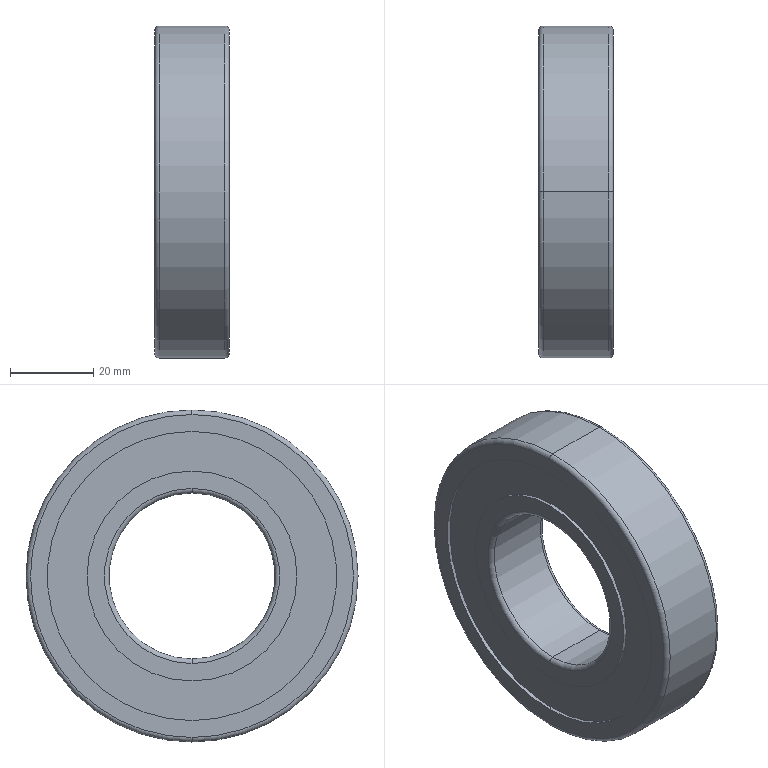Part | SolidWorks | features Fillet 2, Revolution 1 | 1 solid | 26 faces | box 18 x 80 x 80 mm | volume 64676 mm3 | cylinder 12 | torus 8 | plane 6 | commonest cylinder face diameters 50.6 x4 69.65 x4 40 x2 80 x2
STEP:
#1=CARTESIAN_POINT('',(1.1,0.,20.));
#2=VERTEX_POINT('',#1);
#3=CARTESIAN_POINT('',(1.1,0.,-20.));
#4=VERTEX_POINT('',#3);
#5=CARTESIAN_POINT('',(1.1,0.,0.));
#6=DIRECTION('',(-1.,0.,0.));
#7=DIRECTION('',(0.,0.,-1.));
#8=AXIS2_PLACEMENT_3D('',#5,#6,#7);
#9=CIRCLE('',#8,20.);
#10=EDGE_CURVE('',#2,#4,#9,.T.);
#11=ORIENTED_EDGE('',*,*,#10,.F.);
#12=CARTESIAN_POINT('',(0.,0.,21.1));
#13=VERTEX_POINT('',#12);
#14=CARTESIAN_POINT('',(1.1,0.,21.1));
#15=DIRECTION('',(0.,1.,0.));
#16=DIRECTION('',(0.,0.,1.));
#17=AXIS2_PLACEMENT_3D('',#14,#15,#16);
#18=CIRCLE('',#17,1.1);
#19=EDGE_CURVE('',#2,#13,#18,.T.);
#20=ORIENTED_EDGE('',*,*,#19,.T.);
#21=CARTESIAN_POINT('',(0.,0.,-21.1));
#22=VERTEX_POINT('',#21);
#23=CARTESIAN_POINT('',(0.,0.,0.));
#24=DIRECTION('',(1.,0.,0.));
#25=DIRECTION('',(0.,0.,-1.));
#26=AXIS2_PLACEMENT_3D('',#23,#24,#25);
#27=CIRCLE('',#26,21.1);
#28=EDGE_CURVE('',#22,#13,#27,.T.);
#29=ORIENTED_EDGE('',*,*,#28,.F.);
#30=CARTESIAN_POINT('',(1.1,0.,-21.1));
#31=DIRECTION('',(0.,-1.,0.));
#32=DIRECTION('',(0.,0.,-1.));
#33=AXIS2_PLACEMENT_3D('',#30,#31,#32);
#34=CIRCLE('',#33,1.1);
#35=EDGE_CURVE('',#4,#22,#34,.T.);
#36=ORIENTED_EDGE('',*,*,#35,.F.);
#37=EDGE_LOOP('',(#11,#20,#29,#36));
#38=FACE_OUTER_BOUND('',#37,.T.);
#39=CARTESIAN_POINT('',(1.1,0.,0.));
#40=DIRECTION('',(1.,0.,0.));
#41=DIRECTION('',(0.,0.,-1.));
#42=AXIS2_PLACEMENT_3D('',#39,#40,#41);
#43=TOROIDAL_SURFACE('',#42,21.1,1.1);
#44=ADVANCED_FACE('',(#38),#43,.T.);
#45=CARTESIAN_POINT('',(16.9,0.,-20.));
#46=VERTEX_POINT('',#45);
#47=CARTESIAN_POINT('',(16.9,0.,20.));
#48=VERTEX_POINT('',#47);
#49=CARTESIAN_POINT('',(16.9,0.,0.));
#50=DIRECTION('',(1.,0.,0.));
#51=DIRECTION('',(0.,0.,1.));
#52=AXIS2_PLACEMENT_3D('',#49,#50,#51);
#53=CIRCLE('',#52,20.);
#54=EDGE_CURVE('',#46,#48,#53,.T.);
#55=ORIENTED_EDGE('',*,*,#54,.F.);
#56=CARTESIAN_POINT('',(18.,0.,-21.1));
#57=VERTEX_POINT('',#56);
#58=CARTESIAN_POINT('',(16.9,0.,-21.1));
#59=DIRECTION('',(0.,1.,0.));
#60=DIRECTION('',(0.,0.,1.));
#61=AXIS2_PLACEMENT_3D('',#58,#59,#60);
#62=CIRCLE('',#61,1.1);
#63=EDGE_CURVE('',#46,#57,#62,.T.);
#64=ORIENTED_EDGE('',*,*,#63,.T.);
#65=CARTESIAN_POINT('',(18.,0.,21.1));
#66=VERTEX_POINT('',#65);
#67=CARTESIAN_POINT('',(18.,0.,0.));
#68=DIRECTION('',(-1.,0.,0.));
#69=DIRECTION('',(0.,0.,1.));
#70=AXIS2_PLACEMENT_3D('',#67,#68,#69);
#71=CIRCLE('',#70,21.1);
#72=EDGE_CURVE('',#66,#57,#71,.T.);
#73=ORIENTED_EDGE('',*,*,#72,.F.);
#74=CARTESIAN_POINT('',(16.9,0.,21.1));
#75=DIRECTION('',(0.,-1.,0.));
#76=DIRECTION('',(0.,0.,-1.));
#77=AXIS2_PLACEMENT_3D('',#74,#75,#76);
#78=CIRCLE('',#77,1.1);
#79=EDGE_CURVE('',#48,#66,#78,.T.);
#80=ORIENTED_EDGE('',*,*,#79,.F.);
#81=EDGE_LOOP('',(#55,#64,#73,#80));
#82=FACE_OUTER_BOUND('',#81,.T.);
#83=CARTESIAN_POINT('',(16.9,0.,0.));
#84=DIRECTION('',(-1.,0.,0.));
#85=DIRECTION('',(0.,0.,1.));
#86=AXIS2_PLACEMENT_3D('',#83,#84,#85);
#87=TOROIDAL_SURFACE('',#86,21.1,1.1);
#88=ADVANCED_FACE('',(#82),#87,.T.);
#89=CARTESIAN_POINT('',(0.,0.,38.9));
#90=VERTEX_POINT('',#89);
#91=CARTESIAN_POINT('',(0.,0.,-38.9));
#92=VERTEX_POINT('',#91);
#93=CARTESIAN_POINT('',(0.,0.,0.));
#94=DIRECTION('',(-1.,0.,0.));
#95=DIRECTION('',(0.,0.,-1.));
#96=AXIS2_PLACEMENT_3D('',#93,#94,#95);
#97=CIRCLE('',#96,38.9);
#98=EDGE_CURVE('',#90,#92,#97,.T.);
#99=ORIENTED_EDGE('',*,*,#98,.F.);
#100=CARTESIAN_POINT('',(1.1,0.,40.));
#101=VERTEX_POINT('',#100);
#102=CARTESIAN_POINT('',(1.1,0.,38.9));
#103=DIRECTION('',(0.,1.,0.));
#104=DIRECTION('',(0.,0.,1.));
#105=AXIS2_PLACEMENT_3D('',#102,#103,#104);
#106=CIRCLE('',#105,1.1);
#107=EDGE_CURVE('',#90,#101,#106,.T.);
#108=ORIENTED_EDGE('',*,*,#107,.T.);
#109=CARTESIAN_POINT('',(1.1,0.,-40.));
#110=VERTEX_POINT('',#109);
#111=CARTESIAN_POINT('',(1.1,0.,0.));
#112=DIRECTION('',(1.,0.,0.));
#113=DIRECTION('',(0.,0.,-1.));
#114=AXIS2_PLACEMENT_3D('',#111,#112,#113);
#115=CIRCLE('',#114,40.);
#116=EDGE_CURVE('',#110,#101,#115,.T.);
#117=ORIENTED_EDGE('',*,*,#116,.F.);
#118=CARTESIAN_POINT('',(1.1,0.,-38.9));
#119=DIRECTION('',(0.,-1.,0.));
#120=DIRECTION('',(0.,0.,-1.));
#121=AXIS2_PLACEMENT_3D('',#118,#119,#120);
#122=CIRCLE('',#121,1.1);
#123=EDGE_CURVE('',#92,#110,#122,.T.);
#124=ORIENTED_EDGE('',*,*,#123,.F.);
#125=EDGE_LOOP('',(#99,#108,#117,#124));
#126=FACE_OUTER_BOUND('',#125,.T.);
#127=CARTESIAN_POINT('',(1.1,0.,0.));
#128=DIRECTION('',(1.,0.,0.));
#129=DIRECTION('',(0.,0.,-1.));
#130=AXIS2_PLACEMENT_3D('',#127,#128,#129);
#131=TOROIDAL_SURFACE('',#130,38.9,1.1);
#132=ADVANCED_FACE('',(#126),#131,.T.);
#133=CARTESIAN_POINT('',(18.,0.,-38.9));
#134=VERTEX_POINT('',#133);
#135=CARTESIAN_POINT('',(18.,0.,38.9));
#136=VERTEX_POINT('',#135);
#137=CARTESIAN_POINT('',(18.,0.,0.));
#138=DIRECTION('',(1.,0.,0.));
#139=DIRECTION('',(0.,0.,1.));
#140=AXIS2_PLACEMENT_3D('',#137,#138,#139);
#141=CIRCLE('',#140,38.9);
#142=EDGE_CURVE('',#134,#136,#141,.T.);
#143=ORIENTED_EDGE('',*,*,#142,.F.);
#144=CARTESIAN_POINT('',(16.9,0.,-40.));
#145=VERTEX_POINT('',#144);
#146=CARTESIAN_POINT('',(16.9,0.,-38.9));
#147=DIRECTION('',(0.,1.,0.));
#148=DIRECTION('',(0.,0.,1.));
#149=AXIS2_PLACEMENT_3D('',#146,#147,#148);
#150=CIRCLE('',#149,1.1);
#151=EDGE_CURVE('',#134,#145,#150,.T.);
#152=ORIENTED_EDGE('',*,*,#151,.T.);
#153=CARTESIAN_POINT('',(16.9,0.,40.));
#154=VERTEX_POINT('',#153);
#155=CARTESIAN_POINT('',(16.9,0.,0.));
#156=DIRECTION('',(-1.,0.,0.));
#157=DIRECTION('',(0.,0.,1.));
#158=AXIS2_PLACEMENT_3D('',#155,#156,#157);
#159=CIRCLE('',#158,40.);
#160=EDGE_CURVE('',#154,#145,#159,.T.);
#161=ORIENTED_EDGE('',*,*,#160,.F.);
#162=CARTESIAN_POINT('',(16.9,0.,38.9));
#163=DIRECTION('',(0.,-1.,0.));
#164=DIRECTION('',(0.,0.,-1.));
#165=AXIS2_PLACEMENT_3D('',#162,#163,#164);
#166=CIRCLE('',#165,1.1);
#167=EDGE_CURVE('',#136,#154,#166,.T.);
#168=ORIENTED_EDGE('',*,*,#167,.F.);
#169=EDGE_LOOP('',(#143,#152,#161,#168));
#170=FACE_OUTER_BOUND('',#169,.T.);
#171=CARTESIAN_POINT('',(16.9,0.,0.));
#172=DIRECTION('',(-1.,0.,0.));
#173=DIRECTION('',(0.,0.,1.));
#174=AXIS2_PLACEMENT_3D('',#171,#172,#173);
#175=TOROIDAL_SURFACE('',#174,38.9,1.1);
#176=ADVANCED_FACE('',(#170),#175,.T.);
#177=ORIENTED_EDGE('',*,*,#160,.T.);
#178=CARTESIAN_POINT('',(0.,0.,-40.));
#179=DIRECTION('',(-1.,0.,0.));
#180=VECTOR('',#179,1000.);
#181=LINE('',#178,#180);
#182=EDGE_CURVE('',#145,#110,#181,.T.);
#183=ORIENTED_EDGE('',*,*,#182,.T.);
#184=ORIENTED_EDGE('',*,*,#116,.T.);
#185=CARTESIAN_POINT('',(0.,0.,40.));
#186=DIRECTION('',(-1.,0.,0.));
#187=VECTOR('',#186,1000.);
#188=LINE('',#185,#187);
#189=EDGE_CURVE('',#154,#101,#188,.T.);
#190=ORIENTED_EDGE('',*,*,#189,.F.);
#191=EDGE_LOOP('',(#177,#183,#184,#190));
#192=FACE_OUTER_BOUND('',#191,.T.);
#193=CARTESIAN_POINT('',(0.,0.,0.));
#194=DIRECTION('',(-1.,0.,0.));
#195=DIRECTION('',(0.,0.,1.));
#196=AXIS2_PLACEMENT_3D('',#193,#194,#195);
#197=CYLINDRICAL_SURFACE('',#196,40.);
#198=ADVANCED_FACE('',(#192),#197,.T.);
#199=CARTESIAN_POINT('',(18.,0.,-34.825));
#200=VERTEX_POINT('',#199);
#201=CARTESIAN_POINT('',(18.,0.,34.825));
#202=VERTEX_POINT('',#201);
#203=CARTESIAN_POINT('',(18.,0.,0.));
#204=DIRECTION('',(-1.,0.,0.));
#205=DIRECTION('',(0.,0.,1.));
#206=AXIS2_PLACEMENT_3D('',#203,#204,#205);
#207=CIRCLE('',#206,34.825);
#208=EDGE_CURVE('',#200,#202,#207,.T.);
#209=ORIENTED_EDGE('',*,*,#208,.F.);
#210=CARTESIAN_POINT('',(17.17,0.,-34.825));
#211=VERTEX_POINT('',#210);
#212=CARTESIAN_POINT('',(0.,0.,-34.825));
#213=DIRECTION('',(-1.,0.,0.));
#214=VECTOR('',#213,1000.);
#215=LINE('',#212,#214);
#216=EDGE_CURVE('',#200,#211,#215,.T.);
#217=ORIENTED_EDGE('',*,*,#216,.T.);
#218=CARTESIAN_POINT('',(17.17,0.,34.825));
#219=VERTEX_POINT('',#218);
#220=CARTESIAN_POINT('',(17.17,0.,0.));
#221=DIRECTION('',(-1.,0.,0.));
#222=DIRECTION('',(0.,0.,1.));
#223=AXIS2_PLACEMENT_3D('',#220,#221,#222);
#224=CIRCLE('',#223,34.825);
#225=EDGE_CURVE('',#211,#219,#224,.T.);
#226=ORIENTED_EDGE('',*,*,#225,.T.);
#227=CARTESIAN_POINT('',(0.,0.,34.825));
#228=DIRECTION('',(-1.,0.,0.));
#229=VECTOR('',#228,1000.);
#230=LINE('',#227,#229);
#231=EDGE_CURVE('',#202,#219,#230,.T.);
#232=ORIENTED_EDGE('',*,*,#231,.F.);
#233=EDGE_LOOP('',(#209,#217,#226,#232));
#234=FACE_OUTER_BOUND('',#233,.T.);
#235=CARTESIAN_POINT('',(0.,0.,0.));
#236=DIRECTION('',(-1.,0.,0.));
#237=DIRECTION('',(0.,0.,1.));
#238=AXIS2_PLACEMENT_3D('',#235,#236,#237);
#239=CYLINDRICAL_SURFACE('',#238,34.825);
#240=ADVANCED_FACE('',(#234),#239,.F.);
#241=CARTESIAN_POINT('',(18.,0.,25.3));
#242=VERTEX_POINT('',#241);
#243=CARTESIAN_POINT('',(18.,0.,-25.3));
#244=VERTEX_POINT('',#243);
#245=CARTESIAN_POINT('',(18.,0.,0.));
#246=DIRECTION('',(-1.,0.,0.));
#247=DIRECTION('',(0.,0.,1.));
#248=AXIS2_PLACEMENT_3D('',#245,#246,#247);
#249=CIRCLE('',#248,25.3);
#250=EDGE_CURVE('',#242,#244,#249,.T.);
#251=ORIENTED_EDGE('',*,*,#250,.T.);
#252=CARTESIAN_POINT('',(17.17,0.,-25.3));
#253=VERTEX_POINT('',#252);
#254=CARTESIAN_POINT('',(0.,0.,-25.3));
#255=DIRECTION('',(-1.,0.,0.));
#256=VECTOR('',#255,1000.);
#257=LINE('',#254,#256);
#258=EDGE_CURVE('',#244,#253,#257,.T.);
#259=ORIENTED_EDGE('',*,*,#258,.T.);
#260=CARTESIAN_POINT('',(17.17,0.,25.3));
#261=VERTEX_POINT('',#260);
#262=CARTESIAN_POINT('',(17.17,0.,0.));
#263=DIRECTION('',(-1.,0.,0.));
#264=DIRECTION('',(0.,0.,1.));
#265=AXIS2_PLACEMENT_3D('',#262,#263,#264);
#266=CIRCLE('',#265,25.3);
#267=EDGE_CURVE('',#261,#253,#266,.T.);
#268=ORIENTED_EDGE('',*,*,#267,.F.);
#269=CARTESIAN_POINT('',(0.,0.,25.3));
#270=DIRECTION('',(-1.,0.,0.));
#271=VECTOR('',#270,1000.);
#272=LINE('',#269,#271);
#273=EDGE_CURVE('',#242,#261,#272,.T.);
#274=ORIENTED_EDGE('',*,*,#273,.F.);
#275=EDGE_LOOP('',(#251,#259,#268,#274));
#276=FACE_OUTER_BOUND('',#275,.T.);
#277=CARTESIAN_POINT('',(0.,0.,0.));
#278=DIRECTION('',(-1.,0.,0.));
#279=DIRECTION('',(0.,0.,1.));
#280=AXIS2_PLACEMENT_3D('',#277,#278,#279);
#281=CYLINDRICAL_SURFACE('',#280,25.3);
#282=ADVANCED_FACE('',(#276),#281,.T.);
#283=CARTESIAN_POINT('',(16.9,0.,0.));
#284=DIRECTION('',(1.,0.,0.));
#285=DIRECTION('',(0.,0.,1.));
#286=AXIS2_PLACEMENT_3D('',#283,#284,#285);
#287=CIRCLE('',#286,20.);
#288=EDGE_CURVE('',#48,#46,#287,.T.);
#289=ORIENTED_EDGE('',*,*,#288,.T.);
#290=CARTESIAN_POINT('',(0.,0.,-20.));
#291=DIRECTION('',(-1.,0.,0.));
#292=VECTOR('',#291,1000.);
#293=LINE('',#290,#292);
#294=EDGE_CURVE('',#46,#4,#293,.T.);
#295=ORIENTED_EDGE('',*,*,#294,.T.);
#296=CARTESIAN_POINT('',(1.1,0.,0.));
#297=DIRECTION('',(-1.,0.,0.));
#298=DIRECTION('',(0.,0.,-1.));
#299=AXIS2_PLACEMENT_3D('',#296,#297,#298);
#300=CIRCLE('',#299,20.);
#301=EDGE_CURVE('',#4,#2,#300,.T.);
#302=ORIENTED_EDGE('',*,*,#301,.T.);
#303=CARTESIAN_POINT('',(0.,0.,20.));
#304=DIRECTION('',(-1.,0.,0.));
#305=VECTOR('',#304,1000.);
#306=LINE('',#303,#305);
#307=EDGE_CURVE('',#48,#2,#306,.T.);
#308=ORIENTED_EDGE('',*,*,#307,.F.);
#309=EDGE_LOOP('',(#289,#295,#302,#308));
#310=FACE_OUTER_BOUND('',#309,.T.);
#311=CARTESIAN_POINT('',(0.,0.,0.));
#312=DIRECTION('',(-1.,0.,0.));
#313=DIRECTION('',(0.,0.,1.));
#314=AXIS2_PLACEMENT_3D('',#311,#312,#313);
#315=CYLINDRICAL_SURFACE('',#314,20.);
#316=ADVANCED_FACE('',(#310),#315,.F.);
#317=CARTESIAN_POINT('',(0.83,0.,25.3));
#318=VERTEX_POINT('',#317);
#319=CARTESIAN_POINT('',(0.83,0.,-25.3));
#320=VERTEX_POINT('',#319);
#321=CARTESIAN_POINT('',(0.83,0.,0.));
#322=DIRECTION('',(-1.,0.,0.));
#323=DIRECTION('',(0.,0.,1.));
#324=AXIS2_PLACEMENT_3D('',#321,#322,#323);
#325=CIRCLE('',#324,25.3);
#326=EDGE_CURVE('',#318,#320,#325,.T.);
#327=ORIENTED_EDGE('',*,*,#326,.T.);
#328=CARTESIAN_POINT('',(0.,0.,-25.3));
#329=VERTEX_POINT('',#328);
#330=CARTESIAN_POINT('',(0.,0.,-25.3));
#331=DIRECTION('',(-1.,0.,0.));
#332=VECTOR('',#331,1000.);
#333=LINE('',#330,#332);
#334=EDGE_CURVE('',#320,#329,#333,.T.);
#335=ORIENTED_EDGE('',*,*,#334,.T.);
#336=CARTESIAN_POINT('',(0.,0.,25.3));
#337=VERTEX_POINT('',#336);
#338=CARTESIAN_POINT('',(0.,0.,0.));
#339=DIRECTION('',(-1.,0.,0.));
#340=DIRECTION('',(0.,0.,1.));
#341=AXIS2_PLACEMENT_3D('',#338,#339,#340);
#342=CIRCLE('',#341,25.3);
#343=EDGE_CURVE('',#337,#329,#342,.T.);
#344=ORIENTED_EDGE('',*,*,#343,.F.);
#345=CARTESIAN_POINT('',(0.,0.,25.3));
#346=DIRECTION('',(-1.,0.,0.));
#347=VECTOR('',#346,1000.);
#348=LINE('',#345,#347);
#349=EDGE_CURVE('',#318,#337,#348,.T.);
#350=ORIENTED_EDGE('',*,*,#349,.F.);
#351=EDGE_LOOP('',(#327,#335,#344,#350));
#352=FACE_OUTER_BOUND('',#351,.T.);
#353=CARTESIAN_POINT('',(0.,0.,0.));
#354=DIRECTION('',(-1.,0.,0.));
#355=DIRECTION('',(0.,0.,1.));
#356=AXIS2_PLACEMENT_3D('',#353,#354,#355);
#357=CYLINDRICAL_SURFACE('',#356,25.3);
#358=ADVANCED_FACE('',(#352),#357,.T.);
#359=CARTESIAN_POINT('',(0.83,0.,-34.825));
#360=VERTEX_POINT('',#359);
#361=CARTESIAN_POINT('',(0.83,0.,34.825));
#362=VERTEX_POINT('',#361);
#363=CARTESIAN_POINT('',(0.83,0.,0.));
#364=DIRECTION('',(-1.,0.,0.));
#365=DIRECTION('',(0.,0.,1.));
#366=AXIS2_PLACEMENT_3D('',#363,#364,#365);
#367=CIRCLE('',#366,34.825);
#368=EDGE_CURVE('',#360,#362,#367,.T.);
#369=ORIENTED_EDGE('',*,*,#368,.F.);
#370=CARTESIAN_POINT('',(0.,0.,-34.825));
#371=VERTEX_POINT('',#370);
#372=CARTESIAN_POINT('',(0.,0.,-34.825));
#373=DIRECTION('',(-1.,0.,0.));
#374=VECTOR('',#373,1000.);
#375=LINE('',#372,#374);
#376=EDGE_CURVE('',#360,#371,#375,.T.);
#377=ORIENTED_EDGE('',*,*,#376,.T.);
#378=CARTESIAN_POINT('',(0.,0.,34.825));
#379=VERTEX_POINT('',#378);
#380=CARTESIAN_POINT('',(0.,0.,0.));
#381=DIRECTION('',(-1.,0.,0.));
#382=DIRECTION('',(0.,0.,1.));
#383=AXIS2_PLACEMENT_3D('',#380,#381,#382);
#384=CIRCLE('',#383,34.825);
#385=EDGE_CURVE('',#371,#379,#384,.T.);
#386=ORIENTED_EDGE('',*,*,#385,.T.);
#387=CARTESIAN_POINT('',(0.,0.,34.825));
#388=DIRECTION('',(-1.,0.,0.));
#389=VECTOR('',#388,1000.);
#390=LINE('',#387,#389);
#391=EDGE_CURVE('',#362,#379,#390,.T.);
#392=ORIENTED_EDGE('',*,*,#391,.F.);
#393=EDGE_LOOP('',(#369,#377,#386,#392));
#394=FACE_OUTER_BOUND('',#393,.T.);
#395=CARTESIAN_POINT('',(0.,0.,0.));
#396=DIRECTION('',(-1.,0.,0.));
#397=DIRECTION('',(0.,0.,1.));
#398=AXIS2_PLACEMENT_3D('',#395,#396,#397);
#399=CYLINDRICAL_SURFACE('',#398,34.825);
#400=ADVANCED_FACE('',(#394),#399,.F.);
#401=CARTESIAN_POINT('',(0.,0.,0.));
#402=DIRECTION('',(-1.,0.,0.));
#403=DIRECTION('',(0.,0.,-1.));
#404=AXIS2_PLACEMENT_3D('',#401,#402,#403);
#405=CIRCLE('',#404,38.9);
#406=EDGE_CURVE('',#92,#90,#405,.T.);
#407=ORIENTED_EDGE('',*,*,#406,.T.);
#408=ORIENTED_EDGE('',*,*,#98,.T.);
#409=EDGE_LOOP('',(#407,#408));
#410=FACE_OUTER_BOUND('',#409,.T.);
#411=CARTESIAN_POINT('',(0.,0.,0.));
#412=DIRECTION('',(-1.,0.,0.));
#413=DIRECTION('',(0.,0.,1.));
#414=AXIS2_PLACEMENT_3D('',#411,#412,#413);
#415=CIRCLE('',#414,34.825);
#416=EDGE_CURVE('',#379,#371,#415,.T.);
#417=ORIENTED_EDGE('',*,*,#416,.F.);
#418=ORIENTED_EDGE('',*,*,#385,.F.);
#419=EDGE_LOOP('',(#417,#418));
#420=FACE_BOUND('',#419,.T.);
#421=CARTESIAN_POINT('',(0.,40.,0.));
#422=DIRECTION('',(1.,0.,0.));
#423=DIRECTION('',(0.,0.,-1.));
#424=AXIS2_PLACEMENT_3D('',#421,#422,#423);
#425=PLANE('',#424);
#426=ADVANCED_FACE('',(#410,#420),#425,.F.);
#427=ORIENTED_EDGE('',*,*,#376,.F.);
#428=CARTESIAN_POINT('',(0.83,0.,0.));
#429=DIRECTION('',(-1.,0.,0.));
#430=DIRECTION('',(0.,0.,1.));
#431=AXIS2_PLACEMENT_3D('',#428,#429,#430);
#432=CIRCLE('',#431,34.825);
#433=EDGE_CURVE('',#362,#360,#432,.T.);
#434=ORIENTED_EDGE('',*,*,#433,.F.);
#435=ORIENTED_EDGE('',*,*,#391,.T.);
#436=ORIENTED_EDGE('',*,*,#416,.T.);
#437=EDGE_LOOP('',(#427,#434,#435,#436));
#438=FACE_OUTER_BOUND('',#437,.T.);
#439=CARTESIAN_POINT('',(0.,0.,0.));
#440=DIRECTION('',(-1.,0.,0.));
#441=DIRECTION('',(0.,0.,1.));
#442=AXIS2_PLACEMENT_3D('',#439,#440,#441);
#443=CYLINDRICAL_SURFACE('',#442,34.825);
#444=ADVANCED_FACE('',(#438),#443,.F.);
#445=ORIENTED_EDGE('',*,*,#326,.F.);
#446=CARTESIAN_POINT('',(0.83,0.,0.));
#447=DIRECTION('',(-1.,0.,0.));
#448=DIRECTION('',(0.,0.,1.));
#449=AXIS2_PLACEMENT_3D('',#446,#447,#448);
#450=CIRCLE('',#449,25.3);
#451=EDGE_CURVE('',#320,#318,#450,.T.);
#452=ORIENTED_EDGE('',*,*,#451,.F.);
#453=EDGE_LOOP('',(#445,#452));
#454=FACE_BOUND('',#453,.T.);
#455=ORIENTED_EDGE('',*,*,#433,.T.);
#456=ORIENTED_EDGE('',*,*,#368,.T.);
#457=EDGE_LOOP('',(#455,#456));
#458=FACE_OUTER_BOUND('',#457,.T.);
#459=CARTESIAN_POINT('',(0.83,34.825,0.));
#460=DIRECTION('',(1.,0.,0.));
#461=DIRECTION('',(0.,0.,-1.));
#462=AXIS2_PLACEMENT_3D('',#459,#460,#461);
#463=PLANE('',#462);
#464=ADVANCED_FACE('',(#454,#458),#463,.F.);
#465=ORIENTED_EDGE('',*,*,#334,.F.);
#466=ORIENTED_EDGE('',*,*,#451,.T.);
#467=ORIENTED_EDGE('',*,*,#349,.T.);
#468=CARTESIAN_POINT('',(0.,0.,0.));
#469=DIRECTION('',(-1.,0.,0.));
#470=DIRECTION('',(0.,0.,1.));
#471=AXIS2_PLACEMENT_3D('',#468,#469,#470);
#472=CIRCLE('',#471,25.3);
#473=EDGE_CURVE('',#329,#337,#472,.T.);
#474=ORIENTED_EDGE('',*,*,#473,.F.);
#475=EDGE_LOOP('',(#465,#466,#467,#474));
#476=FACE_OUTER_BOUND('',#475,.T.);
#477=CARTESIAN_POINT('',(0.,0.,0.));
#478=DIRECTION('',(-1.,0.,0.));
#479=DIRECTION('',(0.,0.,1.));
#480=AXIS2_PLACEMENT_3D('',#477,#478,#479);
#481=CYLINDRICAL_SURFACE('',#480,25.3);
#482=ADVANCED_FACE('',(#476),#481,.T.);
#483=ORIENTED_EDGE('',*,*,#28,.T.);
#484=CARTESIAN_POINT('',(0.,0.,0.));
#485=DIRECTION('',(1.,0.,0.));
#486=DIRECTION('',(0.,0.,-1.));
#487=AXIS2_PLACEMENT_3D('',#484,#485,#486);
#488=CIRCLE('',#487,21.1);
#489=EDGE_CURVE('',#13,#22,#488,.T.);
#490=ORIENTED_EDGE('',*,*,#489,.T.);
#491=EDGE_LOOP('',(#483,#490));
#492=FACE_BOUND('',#491,.T.);
#493=ORIENTED_EDGE('',*,*,#343,.T.);
#494=ORIENTED_EDGE('',*,*,#473,.T.);
#495=EDGE_LOOP('',(#493,#494));
#496=FACE_OUTER_BOUND('',#495,.T.);
#497=CARTESIAN_POINT('',(0.,25.3,0.));
#498=DIRECTION('',(1.,0.,0.));
#499=DIRECTION('',(0.,0.,-1.));
#500=AXIS2_PLACEMENT_3D('',#497,#498,#499);
#501=PLANE('',#500);
#502=ADVANCED_FACE('',(#492,#496),#501,.F.);
#503=ORIENTED_EDGE('',*,*,#294,.F.);
#504=ORIENTED_EDGE('',*,*,#54,.T.);
#505=ORIENTED_EDGE('',*,*,#307,.T.);
#506=ORIENTED_EDGE('',*,*,#10,.T.);
#507=EDGE_LOOP('',(#503,#504,#505,#506));
#508=FACE_OUTER_BOUND('',#507,.T.);
#509=CARTESIAN_POINT('',(0.,0.,0.));
#510=DIRECTION('',(-1.,0.,0.));
#511=DIRECTION('',(0.,0.,1.));
#512=AXIS2_PLACEMENT_3D('',#509,#510,#511);
#513=CYLINDRICAL_SURFACE('',#512,20.);
#514=ADVANCED_FACE('',(#508),#513,.F.);
#515=ORIENTED_EDGE('',*,*,#72,.T.);
#516=CARTESIAN_POINT('',(18.,0.,0.));
#517=DIRECTION('',(-1.,0.,0.));
#518=DIRECTION('',(0.,0.,1.));
#519=AXIS2_PLACEMENT_3D('',#516,#517,#518);
#520=CIRCLE('',#519,21.1);
#521=EDGE_CURVE('',#57,#66,#520,.T.);
#522=ORIENTED_EDGE('',*,*,#521,.T.);
#523=EDGE_LOOP('',(#515,#522));
#524=FACE_BOUND('',#523,.T.);
#525=ORIENTED_EDGE('',*,*,#250,.F.);
#526=CARTESIAN_POINT('',(18.,0.,0.));
#527=DIRECTION('',(-1.,0.,0.));
#528=DIRECTION('',(0.,0.,1.));
#529=AXIS2_PLACEMENT_3D('',#526,#527,#528);
#530=CIRCLE('',#529,25.3);
#531=EDGE_CURVE('',#244,#242,#530,.T.);
#532=ORIENTED_EDGE('',*,*,#531,.F.);
#533=EDGE_LOOP('',(#525,#532));
#534=FACE_OUTER_BOUND('',#533,.T.);
#535=CARTESIAN_POINT('',(18.,25.3,0.));
#536=DIRECTION('',(-1.,0.,0.));
#537=DIRECTION('',(0.,0.,1.));
#538=AXIS2_PLACEMENT_3D('',#535,#536,#537);
#539=PLANE('',#538);
#540=ADVANCED_FACE('',(#524,#534),#539,.F.);
#541=ORIENTED_EDGE('',*,*,#258,.F.);
#542=ORIENTED_EDGE('',*,*,#531,.T.);
#543=ORIENTED_EDGE('',*,*,#273,.T.);
#544=CARTESIAN_POINT('',(17.17,0.,0.));
#545=DIRECTION('',(-1.,0.,0.));
#546=DIRECTION('',(0.,0.,1.));
#547=AXIS2_PLACEMENT_3D('',#544,#545,#546);
#548=CIRCLE('',#547,25.3);
#549=EDGE_CURVE('',#253,#261,#548,.T.);
#550=ORIENTED_EDGE('',*,*,#549,.F.);
#551=EDGE_LOOP('',(#541,#542,#543,#550));
#552=FACE_OUTER_BOUND('',#551,.T.);
#553=CARTESIAN_POINT('',(0.,0.,0.));
#554=DIRECTION('',(-1.,0.,0.));
#555=DIRECTION('',(0.,0.,1.));
#556=AXIS2_PLACEMENT_3D('',#553,#554,#555);
#557=CYLINDRICAL_SURFACE('',#556,25.3);
#558=ADVANCED_FACE('',(#552),#557,.T.);
#559=CARTESIAN_POINT('',(17.17,0.,0.));
#560=DIRECTION('',(-1.,0.,0.));
#561=DIRECTION('',(0.,0.,1.));
#562=AXIS2_PLACEMENT_3D('',#559,#560,#561);
#563=CIRCLE('',#562,34.825);
#564=EDGE_CURVE('',#219,#211,#563,.T.);
#565=ORIENTED_EDGE('',*,*,#564,.F.);
#566=ORIENTED_EDGE('',*,*,#225,.F.);
#567=EDGE_LOOP('',(#565,#566));
#568=FACE_OUTER_BOUND('',#567,.T.);
#569=ORIENTED_EDGE('',*,*,#267,.T.);
#570=ORIENTED_EDGE('',*,*,#549,.T.);
#571=EDGE_LOOP('',(#569,#570));
#572=FACE_BOUND('',#571,.T.);
#573=CARTESIAN_POINT('',(17.17,34.825,0.));
#574=DIRECTION('',(-1.,0.,0.));
#575=DIRECTION('',(0.,0.,1.));
#576=AXIS2_PLACEMENT_3D('',#573,#574,#575);
#577=PLANE('',#576);
#578=ADVANCED_FACE('',(#568,#572),#577,.F.);
#579=ORIENTED_EDGE('',*,*,#216,.F.);
#580=CARTESIAN_POINT('',(18.,0.,0.));
#581=DIRECTION('',(-1.,0.,0.));
#582=DIRECTION('',(0.,0.,1.));
#583=AXIS2_PLACEMENT_3D('',#580,#581,#582);
#584=CIRCLE('',#583,34.825);
#585=EDGE_CURVE('',#202,#200,#584,.T.);
#586=ORIENTED_EDGE('',*,*,#585,.F.);
#587=ORIENTED_EDGE('',*,*,#231,.T.);
#588=ORIENTED_EDGE('',*,*,#564,.T.);
#589=EDGE_LOOP('',(#579,#586,#587,#588));
#590=FACE_OUTER_BOUND('',#589,.T.);
#591=CARTESIAN_POINT('',(0.,0.,0.));
#592=DIRECTION('',(-1.,0.,0.));
#593=DIRECTION('',(0.,0.,1.));
#594=AXIS2_PLACEMENT_3D('',#591,#592,#593);
#595=CYLINDRICAL_SURFACE('',#594,34.825);
#596=ADVANCED_FACE('',(#590),#595,.F.);
#597=CARTESIAN_POINT('',(18.,0.,0.));
#598=DIRECTION('',(1.,0.,0.));
#599=DIRECTION('',(0.,0.,1.));
#600=AXIS2_PLACEMENT_3D('',#597,#598,#599);
#601=CIRCLE('',#600,38.9);
#602=EDGE_CURVE('',#136,#134,#601,.T.);
#603=ORIENTED_EDGE('',*,*,#602,.T.);
#604=ORIENTED_EDGE('',*,*,#142,.T.);
#605=EDGE_LOOP('',(#603,#604));
#606=FACE_OUTER_BOUND('',#605,.T.);
#607=ORIENTED_EDGE('',*,*,#585,.T.);
#608=ORIENTED_EDGE('',*,*,#208,.T.);
#609=EDGE_LOOP('',(#607,#608));
#610=FACE_BOUND('',#609,.T.);
#611=CARTESIAN_POINT('',(18.,40.,0.));
#612=DIRECTION('',(-1.,0.,0.));
#613=DIRECTION('',(0.,0.,1.));
#614=AXIS2_PLACEMENT_3D('',#611,#612,#613);
#615=PLANE('',#614);
#616=ADVANCED_FACE('',(#606,#610),#615,.F.);
#617=ORIENTED_EDGE('',*,*,#182,.F.);
#618=CARTESIAN_POINT('',(16.9,0.,0.));
#619=DIRECTION('',(-1.,0.,0.));
#620=DIRECTION('',(0.,0.,1.));
#621=AXIS2_PLACEMENT_3D('',#618,#619,#620);
#622=CIRCLE('',#621,40.);
#623=EDGE_CURVE('',#145,#154,#622,.T.);
#624=ORIENTED_EDGE('',*,*,#623,.T.);
#625=ORIENTED_EDGE('',*,*,#189,.T.);
#626=CARTESIAN_POINT('',(1.1,0.,0.));
#627=DIRECTION('',(1.,0.,0.));
#628=DIRECTION('',(0.,0.,-1.));
#629=AXIS2_PLACEMENT_3D('',#626,#627,#628);
#630=CIRCLE('',#629,40.);
#631=EDGE_CURVE('',#101,#110,#630,.T.);
#632=ORIENTED_EDGE('',*,*,#631,.T.);
#633=EDGE_LOOP('',(#617,#624,#625,#632));
#634=FACE_OUTER_BOUND('',#633,.T.);
#635=CARTESIAN_POINT('',(0.,0.,0.));
#636=DIRECTION('',(-1.,0.,0.));
#637=DIRECTION('',(0.,0.,1.));
#638=AXIS2_PLACEMENT_3D('',#635,#636,#637);
#639=CYLINDRICAL_SURFACE('',#638,40.);
#640=ADVANCED_FACE('',(#634),#639,.T.);
#641=ORIENTED_EDGE('',*,*,#151,.F.);
#642=ORIENTED_EDGE('',*,*,#602,.F.);
#643=ORIENTED_EDGE('',*,*,#167,.T.);
#644=ORIENTED_EDGE('',*,*,#623,.F.);
#645=EDGE_LOOP('',(#641,#642,#643,#644));
#646=FACE_OUTER_BOUND('',#645,.T.);
#647=CARTESIAN_POINT('',(16.9,0.,0.));
#648=DIRECTION('',(-1.,0.,0.));
#649=DIRECTION('',(0.,0.,1.));
#650=AXIS2_PLACEMENT_3D('',#647,#648,#649);
#651=TOROIDAL_SURFACE('',#650,38.9,1.1);
#652=ADVANCED_FACE('',(#646),#651,.T.);
#653=ORIENTED_EDGE('',*,*,#107,.F.);
#654=ORIENTED_EDGE('',*,*,#406,.F.);
#655=ORIENTED_EDGE('',*,*,#123,.T.);
#656=ORIENTED_EDGE('',*,*,#631,.F.);
#657=EDGE_LOOP('',(#653,#654,#655,#656));
#658=FACE_OUTER_BOUND('',#657,.T.);
#659=CARTESIAN_POINT('',(1.1,0.,0.));
#660=DIRECTION('',(1.,0.,0.));
#661=DIRECTION('',(0.,0.,-1.));
#662=AXIS2_PLACEMENT_3D('',#659,#660,#661);
#663=TOROIDAL_SURFACE('',#662,38.9,1.1);
#664=ADVANCED_FACE('',(#658),#663,.T.);
#665=ORIENTED_EDGE('',*,*,#63,.F.);
#666=ORIENTED_EDGE('',*,*,#288,.F.);
#667=ORIENTED_EDGE('',*,*,#79,.T.);
#668=ORIENTED_EDGE('',*,*,#521,.F.);
#669=EDGE_LOOP('',(#665,#666,#667,#668));
#670=FACE_OUTER_BOUND('',#669,.T.);
#671=CARTESIAN_POINT('',(16.9,0.,0.));
#672=DIRECTION('',(-1.,0.,0.));
#673=DIRECTION('',(0.,0.,1.));
#674=AXIS2_PLACEMENT_3D('',#671,#672,#673);
#675=TOROIDAL_SURFACE('',#674,21.1,1.1);
#676=ADVANCED_FACE('',(#670),#675,.T.);
#677=ORIENTED_EDGE('',*,*,#19,.F.);
#678=ORIENTED_EDGE('',*,*,#301,.F.);
#679=ORIENTED_EDGE('',*,*,#35,.T.);
#680=ORIENTED_EDGE('',*,*,#489,.F.);
#681=EDGE_LOOP('',(#677,#678,#679,#680));
#682=FACE_OUTER_BOUND('',#681,.T.);
#683=CARTESIAN_POINT('',(1.1,0.,0.));
#684=DIRECTION('',(1.,0.,0.));
#685=DIRECTION('',(0.,0.,-1.));
#686=AXIS2_PLACEMENT_3D('',#683,#684,#685);
#687=TOROIDAL_SURFACE('',#686,21.1,1.1);
#688=ADVANCED_FACE('',(#682),#687,.T.);
#689=CLOSED_SHELL('',(#44,#88,#132,#176,#198,#240,#282,#316,#358,#400,#426,#444,#464,#482,#502,#514,#540,#558,#578,#596,#616,#640,#652,#664,#676,#688));
#690=MANIFOLD_SOLID_BREP('',#689);
#691=CARTESIAN_POINT('',(0.,0.,0.));
#692=DIRECTION('',(0.,0.,1.));
#693=DIRECTION('',(1.,0.,0.));
#694=AXIS2_PLACEMENT_3D('',#691,#692,#693);
#695=(LENGTH_UNIT()NAMED_UNIT(*)SI_UNIT(.MILLI.,.METRE.));
#696=UNCERTAINTY_MEASURE_WITH_UNIT(LENGTH_MEASURE(0.00001),#695,'','');
#697=(NAMED_UNIT(*)PLANE_ANGLE_UNIT()SI_UNIT($,.RADIAN.));
#698=(NAMED_UNIT(*)SI_UNIT($,.STERADIAN.)SOLID_ANGLE_UNIT());
#699=(GEOMETRIC_REPRESENTATION_CONTEXT(3)GLOBAL_UNCERTAINTY_ASSIGNED_CONTEXT((#696))GLOBAL_UNIT_ASSIGNED_CONTEXT((#695,#697,#698))REPRESENTATION_CONTEXT('',''));
#700=ADVANCED_BREP_SHAPE_REPRESENTATION('',(#690,#694),#699);